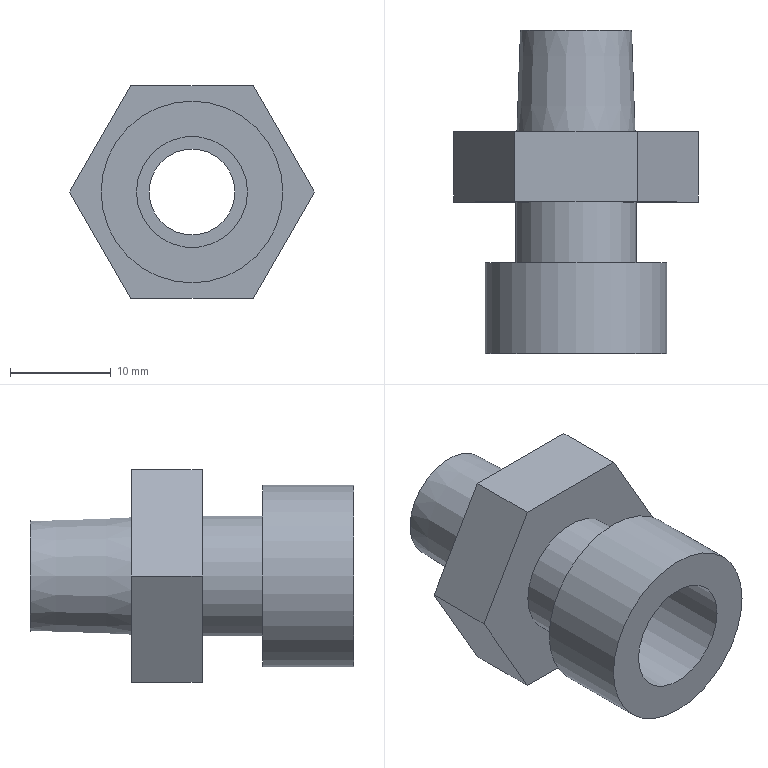Part | NX | features solid 2 | 1 solid | 17 faces | box 24.249 x 32 x 21 mm | volume 4073 mm3 | plane 12 | cylinder 4 | cone 1 | commonest cylinder face diameters 8.5 x1 11 x1 12 x1 18 x1
STEP:
#1=CARTESIAN_POINT('',(25.938,-290.,338.));
#2=VERTEX_POINT('',#1);
#3=CARTESIAN_POINT('',(19.876,-290.,327.5));
#4=VERTEX_POINT('',#3);
#5=CARTESIAN_POINT('',(25.938,-290.,338.));
#6=DIRECTION('',(-0.5,0.,-0.866));
#7=VECTOR('',#6,1000.);
#8=LINE('',#5,#7);
#9=EDGE_CURVE('',#2,#4,#8,.T.);
#10=ORIENTED_EDGE('',*,*,#9,.T.);
#11=CARTESIAN_POINT('',(19.876,-297.,327.5));
#12=VERTEX_POINT('',#11);
#13=CARTESIAN_POINT('',(19.876,-296.,327.5));
#14=DIRECTION('',(0.,1.,0.));
#15=VECTOR('',#14,1000.);
#16=LINE('',#13,#15);
#17=EDGE_CURVE('',#12,#4,#16,.T.);
#18=ORIENTED_EDGE('',*,*,#17,.F.);
#19=CARTESIAN_POINT('',(25.938,-297.,338.));
#20=VERTEX_POINT('',#19);
#21=CARTESIAN_POINT('',(19.876,-297.,327.5));
#22=DIRECTION('',(-0.5,0.,-0.866));
#23=VECTOR('',#22,1000.);
#24=LINE('',#21,#23);
#25=EDGE_CURVE('',#20,#12,#24,.T.);
#26=ORIENTED_EDGE('',*,*,#25,.F.);
#27=CARTESIAN_POINT('',(25.938,-296.,338.));
#28=DIRECTION('',(0.,1.,0.));
#29=VECTOR('',#28,1000.);
#30=LINE('',#27,#29);
#31=EDGE_CURVE('',#20,#2,#30,.T.);
#32=ORIENTED_EDGE('',*,*,#31,.T.);
#33=EDGE_LOOP('',(#10,#18,#26,#32));
#34=FACE_BOUND('',#33,.T.);
#35=CARTESIAN_POINT('',(25.938,-296.,338.));
#36=DIRECTION('',(-0.866,0.,0.5));
#37=DIRECTION('',(-0.5,0.,-0.866));
#38=AXIS2_PLACEMENT_3D('',#35,#36,#37);
#39=PLANE('',#38);
#40=ADVANCED_FACE('',(#34),#39,.T.);
#41=CARTESIAN_POINT('',(25.938,-290.,317.));
#42=VERTEX_POINT('',#41);
#43=CARTESIAN_POINT('',(19.876,-290.,327.5));
#44=DIRECTION('',(0.5,0.,-0.866));
#45=VECTOR('',#44,1000.);
#46=LINE('',#43,#45);
#47=EDGE_CURVE('',#4,#42,#46,.T.);
#48=ORIENTED_EDGE('',*,*,#47,.T.);
#49=CARTESIAN_POINT('',(25.938,-297.,317.));
#50=VERTEX_POINT('',#49);
#51=CARTESIAN_POINT('',(25.938,-296.,317.));
#52=DIRECTION('',(0.,1.,0.));
#53=VECTOR('',#52,1000.);
#54=LINE('',#51,#53);
#55=EDGE_CURVE('',#50,#42,#54,.T.);
#56=ORIENTED_EDGE('',*,*,#55,.F.);
#57=CARTESIAN_POINT('',(19.876,-297.,327.5));
#58=DIRECTION('',(0.5,0.,-0.866));
#59=VECTOR('',#58,1000.);
#60=LINE('',#57,#59);
#61=EDGE_CURVE('',#12,#50,#60,.T.);
#62=ORIENTED_EDGE('',*,*,#61,.F.);
#63=ORIENTED_EDGE('',*,*,#17,.T.);
#64=EDGE_LOOP('',(#48,#56,#62,#63));
#65=FACE_BOUND('',#64,.T.);
#66=CARTESIAN_POINT('',(19.876,-296.,327.5));
#67=DIRECTION('',(-0.866,0.,-0.5));
#68=DIRECTION('',(0.5,0.,-0.866));
#69=AXIS2_PLACEMENT_3D('',#66,#67,#68);
#70=PLANE('',#69);
#71=ADVANCED_FACE('',(#65),#70,.T.);
#72=CARTESIAN_POINT('',(38.062,-290.,317.));
#73=VERTEX_POINT('',#72);
#74=CARTESIAN_POINT('',(25.938,-290.,317.));
#75=DIRECTION('',(1.,0.,0.));
#76=VECTOR('',#75,1000.);
#77=LINE('',#74,#76);
#78=EDGE_CURVE('',#42,#73,#77,.T.);
#79=ORIENTED_EDGE('',*,*,#78,.T.);
#80=CARTESIAN_POINT('',(38.062,-297.,317.));
#81=VERTEX_POINT('',#80);
#82=CARTESIAN_POINT('',(38.062,-296.,317.));
#83=DIRECTION('',(0.,1.,0.));
#84=VECTOR('',#83,1000.);
#85=LINE('',#82,#84);
#86=EDGE_CURVE('',#81,#73,#85,.T.);
#87=ORIENTED_EDGE('',*,*,#86,.F.);
#88=CARTESIAN_POINT('',(19.876,-297.,317.));
#89=DIRECTION('',(1.,0.,0.));
#90=VECTOR('',#89,1000.);
#91=LINE('',#88,#90);
#92=EDGE_CURVE('',#50,#81,#91,.T.);
#93=ORIENTED_EDGE('',*,*,#92,.F.);
#94=ORIENTED_EDGE('',*,*,#55,.T.);
#95=EDGE_LOOP('',(#79,#87,#93,#94));
#96=FACE_BOUND('',#95,.T.);
#97=CARTESIAN_POINT('',(25.938,-296.,317.));
#98=DIRECTION('',(0.,0.,-1.));
#99=DIRECTION('',(1.,0.,0.));
#100=AXIS2_PLACEMENT_3D('',#97,#98,#99);
#101=PLANE('',#100);
#102=ADVANCED_FACE('',(#96),#101,.T.);
#103=CARTESIAN_POINT('',(44.124,-290.,327.5));
#104=VERTEX_POINT('',#103);
#105=CARTESIAN_POINT('',(38.062,-290.,317.));
#106=DIRECTION('',(0.5,0.,0.866));
#107=VECTOR('',#106,1000.);
#108=LINE('',#105,#107);
#109=EDGE_CURVE('',#73,#104,#108,.T.);
#110=ORIENTED_EDGE('',*,*,#109,.T.);
#111=CARTESIAN_POINT('',(44.124,-297.,327.5));
#112=VERTEX_POINT('',#111);
#113=CARTESIAN_POINT('',(44.124,-296.,327.5));
#114=DIRECTION('',(0.,1.,0.));
#115=VECTOR('',#114,1000.);
#116=LINE('',#113,#115);
#117=EDGE_CURVE('',#112,#104,#116,.T.);
#118=ORIENTED_EDGE('',*,*,#117,.F.);
#119=CARTESIAN_POINT('',(38.062,-297.,317.));
#120=DIRECTION('',(0.5,0.,0.866));
#121=VECTOR('',#120,1000.);
#122=LINE('',#119,#121);
#123=EDGE_CURVE('',#81,#112,#122,.T.);
#124=ORIENTED_EDGE('',*,*,#123,.F.);
#125=ORIENTED_EDGE('',*,*,#86,.T.);
#126=EDGE_LOOP('',(#110,#118,#124,#125));
#127=FACE_BOUND('',#126,.T.);
#128=CARTESIAN_POINT('',(38.062,-296.,317.));
#129=DIRECTION('',(0.866,0.,-0.5));
#130=DIRECTION('',(0.5,0.,0.866));
#131=AXIS2_PLACEMENT_3D('',#128,#129,#130);
#132=PLANE('',#131);
#133=ADVANCED_FACE('',(#127),#132,.T.);
#134=CARTESIAN_POINT('',(38.062,-290.,338.));
#135=VERTEX_POINT('',#134);
#136=CARTESIAN_POINT('',(44.124,-290.,327.5));
#137=DIRECTION('',(-0.5,0.,0.866));
#138=VECTOR('',#137,1000.);
#139=LINE('',#136,#138);
#140=EDGE_CURVE('',#104,#135,#139,.T.);
#141=ORIENTED_EDGE('',*,*,#140,.T.);
#142=CARTESIAN_POINT('',(38.062,-297.,338.));
#143=VERTEX_POINT('',#142);
#144=CARTESIAN_POINT('',(38.062,-296.,338.));
#145=DIRECTION('',(0.,1.,0.));
#146=VECTOR('',#145,1000.);
#147=LINE('',#144,#146);
#148=EDGE_CURVE('',#143,#135,#147,.T.);
#149=ORIENTED_EDGE('',*,*,#148,.F.);
#150=CARTESIAN_POINT('',(38.062,-297.,338.));
#151=DIRECTION('',(-0.5,0.,0.866));
#152=VECTOR('',#151,1000.);
#153=LINE('',#150,#152);
#154=EDGE_CURVE('',#112,#143,#153,.T.);
#155=ORIENTED_EDGE('',*,*,#154,.F.);
#156=ORIENTED_EDGE('',*,*,#117,.T.);
#157=EDGE_LOOP('',(#141,#149,#155,#156));
#158=FACE_BOUND('',#157,.T.);
#159=CARTESIAN_POINT('',(44.124,-296.,327.5));
#160=DIRECTION('',(0.866,0.,0.5));
#161=DIRECTION('',(-0.5,0.,0.866));
#162=AXIS2_PLACEMENT_3D('',#159,#160,#161);
#163=PLANE('',#162);
#164=ADVANCED_FACE('',(#158),#163,.T.);
#165=CARTESIAN_POINT('',(38.062,-290.,338.));
#166=DIRECTION('',(-1.,0.,0.));
#167=VECTOR('',#166,1000.);
#168=LINE('',#165,#167);
#169=EDGE_CURVE('',#135,#2,#168,.T.);
#170=ORIENTED_EDGE('',*,*,#169,.T.);
#171=ORIENTED_EDGE('',*,*,#31,.F.);
#172=CARTESIAN_POINT('',(19.876,-297.,338.));
#173=DIRECTION('',(-1.,0.,0.));
#174=VECTOR('',#173,1000.);
#175=LINE('',#172,#174);
#176=EDGE_CURVE('',#143,#20,#175,.T.);
#177=ORIENTED_EDGE('',*,*,#176,.F.);
#178=ORIENTED_EDGE('',*,*,#148,.T.);
#179=EDGE_LOOP('',(#170,#171,#177,#178));
#180=FACE_BOUND('',#179,.T.);
#181=CARTESIAN_POINT('',(38.062,-296.,338.));
#182=DIRECTION('',(0.,0.,1.));
#183=DIRECTION('',(-1.,0.,0.));
#184=AXIS2_PLACEMENT_3D('',#181,#182,#183);
#185=PLANE('',#184);
#186=ADVANCED_FACE('',(#180),#185,.T.);
#187=ORIENTED_EDGE('',*,*,#61,.T.);
#188=ORIENTED_EDGE('',*,*,#92,.T.);
#189=ORIENTED_EDGE('',*,*,#123,.T.);
#190=ORIENTED_EDGE('',*,*,#154,.T.);
#191=ORIENTED_EDGE('',*,*,#176,.T.);
#192=ORIENTED_EDGE('',*,*,#25,.T.);
#193=EDGE_LOOP('',(#187,#188,#189,#190,#191,#192));
#194=FACE_BOUND('',#193,.T.);
#195=CARTESIAN_POINT('',(26.,-297.,327.5));
#196=VERTEX_POINT('',#195);
#197=CARTESIAN_POINT('',(32.,-297.,327.5));
#198=DIRECTION('',(0.,-1.,0.));
#199=DIRECTION('',(-1.,0.,0.));
#200=AXIS2_PLACEMENT_3D('',#197,#198,#199);
#201=CIRCLE('',#200,6.);
#202=EDGE_CURVE('',#196,#196,#201,.F.);
#203=ORIENTED_EDGE('',*,*,#202,.T.);
#204=EDGE_LOOP('',(#203));
#205=FACE_BOUND('',#204,.T.);
#206=CARTESIAN_POINT('',(19.876,-297.,327.5));
#207=DIRECTION('',(0.,1.,0.));
#208=DIRECTION('',(-1.,0.,0.));
#209=AXIS2_PLACEMENT_3D('',#206,#207,#208);
#210=PLANE('',#209);
#211=ADVANCED_FACE('',(#194,#205),#210,.F.);
#212=CARTESIAN_POINT('',(26.151,-290.,327.5));
#213=VERTEX_POINT('',#212);
#214=CARTESIAN_POINT('',(32.,-290.,327.5));
#215=DIRECTION('',(0.,-1.,0.));
#216=DIRECTION('',(-1.,0.,0.));
#217=AXIS2_PLACEMENT_3D('',#214,#215,#216);
#218=CIRCLE('',#217,5.849);
#219=EDGE_CURVE('',#213,#213,#218,.T.);
#220=ORIENTED_EDGE('',*,*,#219,.T.);
#221=EDGE_LOOP('',(#220));
#222=FACE_BOUND('',#221,.T.);
#223=ORIENTED_EDGE('',*,*,#9,.F.);
#224=ORIENTED_EDGE('',*,*,#169,.F.);
#225=ORIENTED_EDGE('',*,*,#140,.F.);
#226=ORIENTED_EDGE('',*,*,#109,.F.);
#227=ORIENTED_EDGE('',*,*,#78,.F.);
#228=ORIENTED_EDGE('',*,*,#47,.F.);
#229=EDGE_LOOP('',(#223,#224,#225,#226,#227,#228));
#230=FACE_BOUND('',#229,.T.);
#231=CARTESIAN_POINT('',(19.876,-290.,327.5));
#232=DIRECTION('',(0.,1.,0.));
#233=DIRECTION('',(-1.,0.,0.));
#234=AXIS2_PLACEMENT_3D('',#231,#232,#233);
#235=PLANE('',#234);
#236=ADVANCED_FACE('',(#222,#230),#235,.T.);
#237=CARTESIAN_POINT('',(36.25,-280.,327.5));
#238=VERTEX_POINT('',#237);
#239=CARTESIAN_POINT('',(32.,-280.,327.5));
#240=DIRECTION('',(0.,1.,0.));
#241=DIRECTION('',(1.,0.,0.));
#242=AXIS2_PLACEMENT_3D('',#239,#240,#241);
#243=CIRCLE('',#242,4.25);
#244=EDGE_CURVE('',#238,#238,#243,.T.);
#245=ORIENTED_EDGE('',*,*,#244,.F.);
#246=EDGE_LOOP('',(#245));
#247=FACE_BOUND('',#246,.T.);
#248=CARTESIAN_POINT('',(26.5,-280.,327.5));
#249=VERTEX_POINT('',#248);
#250=CARTESIAN_POINT('',(32.,-280.,327.5));
#251=DIRECTION('',(0.,-1.,0.));
#252=DIRECTION('',(-1.,0.,0.));
#253=AXIS2_PLACEMENT_3D('',#250,#251,#252);
#254=CIRCLE('',#253,5.5);
#255=EDGE_CURVE('',#249,#249,#254,.T.);
#256=ORIENTED_EDGE('',*,*,#255,.F.);
#257=EDGE_LOOP('',(#256));
#258=FACE_BOUND('',#257,.T.);
#259=CARTESIAN_POINT('',(32.,-280.,327.5));
#260=DIRECTION('',(0.,1.,0.));
#261=DIRECTION('',(-1.,0.,0.));
#262=AXIS2_PLACEMENT_3D('',#259,#260,#261);
#263=PLANE('',#262);
#264=ADVANCED_FACE('',(#247,#258),#263,.T.);
#265=ORIENTED_EDGE('',*,*,#255,.T.);
#266=EDGE_LOOP('',(#265));
#267=FACE_BOUND('',#266,.T.);
#268=ORIENTED_EDGE('',*,*,#219,.F.);
#269=EDGE_LOOP('',(#268));
#270=FACE_BOUND('',#269,.T.);
#271=CARTESIAN_POINT('',(32.,-280.,327.5));
#272=DIRECTION('',(0.,-1.,0.));
#273=DIRECTION('',(-1.,0.,0.));
#274=AXIS2_PLACEMENT_3D('',#271,#272,#273);
#275=CONICAL_SURFACE('',#274,5.5,0.03491);
#276=ADVANCED_FACE('',(#267,#270),#275,.T.);
#277=CARTESIAN_POINT('',(26.5,-312.,327.5));
#278=VERTEX_POINT('',#277);
#279=CARTESIAN_POINT('',(32.,-312.,327.5));
#280=DIRECTION('',(0.,-1.,0.));
#281=DIRECTION('',(-1.,0.,0.));
#282=AXIS2_PLACEMENT_3D('',#279,#280,#281);
#283=CIRCLE('',#282,5.5);
#284=EDGE_CURVE('',#278,#278,#283,.T.);
#285=ORIENTED_EDGE('',*,*,#284,.F.);
#286=EDGE_LOOP('',(#285));
#287=FACE_BOUND('',#286,.T.);
#288=CARTESIAN_POINT('',(41.,-312.,327.5));
#289=VERTEX_POINT('',#288);
#290=CARTESIAN_POINT('',(32.,-312.,327.5));
#291=DIRECTION('',(0.,1.,0.));
#292=DIRECTION('',(1.,0.,0.));
#293=AXIS2_PLACEMENT_3D('',#290,#291,#292);
#294=CIRCLE('',#293,9.);
#295=EDGE_CURVE('',#289,#289,#294,.T.);
#296=ORIENTED_EDGE('',*,*,#295,.F.);
#297=EDGE_LOOP('',(#296));
#298=FACE_BOUND('',#297,.T.);
#299=CARTESIAN_POINT('',(32.,-312.,327.5));
#300=DIRECTION('',(0.,-1.,0.));
#301=DIRECTION('',(1.,0.,0.));
#302=AXIS2_PLACEMENT_3D('',#299,#300,#301);
#303=PLANE('',#302);
#304=ADVANCED_FACE('',(#287,#298),#303,.T.);
#305=CARTESIAN_POINT('',(23.,-303.,327.5));
#306=VERTEX_POINT('',#305);
#307=CARTESIAN_POINT('',(32.,-303.,327.5));
#308=DIRECTION('',(0.,-1.,0.));
#309=DIRECTION('',(-1.,0.,0.));
#310=AXIS2_PLACEMENT_3D('',#307,#308,#309);
#311=CIRCLE('',#310,9.);
#312=EDGE_CURVE('',#306,#306,#311,.T.);
#313=ORIENTED_EDGE('',*,*,#312,.T.);
#314=EDGE_LOOP('',(#313));
#315=FACE_BOUND('',#314,.T.);
#316=ORIENTED_EDGE('',*,*,#295,.T.);
#317=EDGE_LOOP('',(#316));
#318=FACE_BOUND('',#317,.T.);
#319=CARTESIAN_POINT('',(32.,-296.,327.5));
#320=DIRECTION('',(0.,-1.,0.));
#321=DIRECTION('',(1.,0.,0.));
#322=AXIS2_PLACEMENT_3D('',#319,#320,#321);
#323=CYLINDRICAL_SURFACE('',#322,9.);
#324=ADVANCED_FACE('',(#315,#318),#323,.T.);
#325=CARTESIAN_POINT('',(27.75,-292.,327.5));
#326=VERTEX_POINT('',#325);
#327=CARTESIAN_POINT('',(32.,-292.,327.5));
#328=DIRECTION('',(0.,-1.,0.));
#329=DIRECTION('',(-1.,0.,0.));
#330=AXIS2_PLACEMENT_3D('',#327,#328,#329);
#331=CIRCLE('',#330,4.25);
#332=EDGE_CURVE('',#326,#326,#331,.F.);
#333=ORIENTED_EDGE('',*,*,#332,.F.);
#334=EDGE_LOOP('',(#333));
#335=FACE_BOUND('',#334,.T.);
#336=ORIENTED_EDGE('',*,*,#244,.T.);
#337=EDGE_LOOP('',(#336));
#338=FACE_BOUND('',#337,.T.);
#339=CARTESIAN_POINT('',(32.,-280.,327.5));
#340=DIRECTION('',(0.,-1.,0.));
#341=DIRECTION('',(1.,0.,0.));
#342=AXIS2_PLACEMENT_3D('',#339,#340,#341);
#343=CYLINDRICAL_SURFACE('',#342,4.25);
#344=ADVANCED_FACE('',(#335,#338),#343,.F.);
#345=ORIENTED_EDGE('',*,*,#312,.F.);
#346=EDGE_LOOP('',(#345));
#347=FACE_BOUND('',#346,.T.);
#348=CARTESIAN_POINT('',(26.,-303.,327.5));
#349=VERTEX_POINT('',#348);
#350=CARTESIAN_POINT('',(32.,-303.,327.5));
#351=DIRECTION('',(0.,-1.,0.));
#352=DIRECTION('',(-1.,0.,0.));
#353=AXIS2_PLACEMENT_3D('',#350,#351,#352);
#354=CIRCLE('',#353,6.);
#355=EDGE_CURVE('',#349,#349,#354,.F.);
#356=ORIENTED_EDGE('',*,*,#355,.F.);
#357=EDGE_LOOP('',(#356));
#358=FACE_BOUND('',#357,.T.);
#359=CARTESIAN_POINT('',(32.,-303.,327.5));
#360=DIRECTION('',(0.,1.,0.));
#361=DIRECTION('',(-1.,0.,0.));
#362=AXIS2_PLACEMENT_3D('',#359,#360,#361);
#363=PLANE('',#362);
#364=ADVANCED_FACE('',(#347,#358),#363,.T.);
#365=ORIENTED_EDGE('',*,*,#202,.F.);
#366=EDGE_LOOP('',(#365));
#367=FACE_BOUND('',#366,.T.);
#368=ORIENTED_EDGE('',*,*,#355,.T.);
#369=EDGE_LOOP('',(#368));
#370=FACE_BOUND('',#369,.T.);
#371=CARTESIAN_POINT('',(32.,-307.,327.5));
#372=DIRECTION('',(0.,1.,0.));
#373=DIRECTION('',(-1.,0.,0.));
#374=AXIS2_PLACEMENT_3D('',#371,#372,#373);
#375=CYLINDRICAL_SURFACE('',#374,6.);
#376=ADVANCED_FACE('',(#367,#370),#375,.T.);
#377=CARTESIAN_POINT('',(26.5,-292.,327.5));
#378=VERTEX_POINT('',#377);
#379=CARTESIAN_POINT('',(32.,-292.,327.5));
#380=DIRECTION('',(0.,-1.,0.));
#381=DIRECTION('',(-1.,0.,0.));
#382=AXIS2_PLACEMENT_3D('',#379,#380,#381);
#383=CIRCLE('',#382,5.5);
#384=EDGE_CURVE('',#378,#378,#383,.T.);
#385=ORIENTED_EDGE('',*,*,#384,.T.);
#386=EDGE_LOOP('',(#385));
#387=FACE_BOUND('',#386,.T.);
#388=ORIENTED_EDGE('',*,*,#332,.T.);
#389=EDGE_LOOP('',(#388));
#390=FACE_BOUND('',#389,.T.);
#391=CARTESIAN_POINT('',(32.,-292.,327.5));
#392=DIRECTION('',(0.,1.,0.));
#393=DIRECTION('',(-1.,0.,0.));
#394=AXIS2_PLACEMENT_3D('',#391,#392,#393);
#395=PLANE('',#394);
#396=ADVANCED_FACE('',(#387,#390),#395,.F.);
#397=ORIENTED_EDGE('',*,*,#384,.F.);
#398=EDGE_LOOP('',(#397));
#399=FACE_BOUND('',#398,.T.);
#400=ORIENTED_EDGE('',*,*,#284,.T.);
#401=EDGE_LOOP('',(#400));
#402=FACE_BOUND('',#401,.T.);
#403=CARTESIAN_POINT('',(32.,-312.,327.5));
#404=DIRECTION('',(0.,1.,0.));
#405=DIRECTION('',(-1.,0.,0.));
#406=AXIS2_PLACEMENT_3D('',#403,#404,#405);
#407=CYLINDRICAL_SURFACE('',#406,5.5);
#408=ADVANCED_FACE('',(#399,#402),#407,.F.);
#409=CLOSED_SHELL('',(#40,#71,#102,#133,#164,#186,#211,#236,#264,#276,#304,#324,#344,#364,#376,#396,#408));
#410=MANIFOLD_SOLID_BREP('',#409);
#411=(LENGTH_UNIT()NAMED_UNIT(*)SI_UNIT(.MILLI.,.METRE.));
#412=UNCERTAINTY_MEASURE_WITH_UNIT(LENGTH_MEASURE(0.00001),#411,'','');
#413=(NAMED_UNIT(*)PLANE_ANGLE_UNIT()SI_UNIT($,.RADIAN.));
#414=(NAMED_UNIT(*)SI_UNIT($,.STERADIAN.)SOLID_ANGLE_UNIT());
#415=(GEOMETRIC_REPRESENTATION_CONTEXT(3)GLOBAL_UNCERTAINTY_ASSIGNED_CONTEXT((#412))GLOBAL_UNIT_ASSIGNED_CONTEXT((#411,#413,#414))REPRESENTATION_CONTEXT('',''));
#416=ADVANCED_BREP_SHAPE_REPRESENTATION('',(#410),#415);